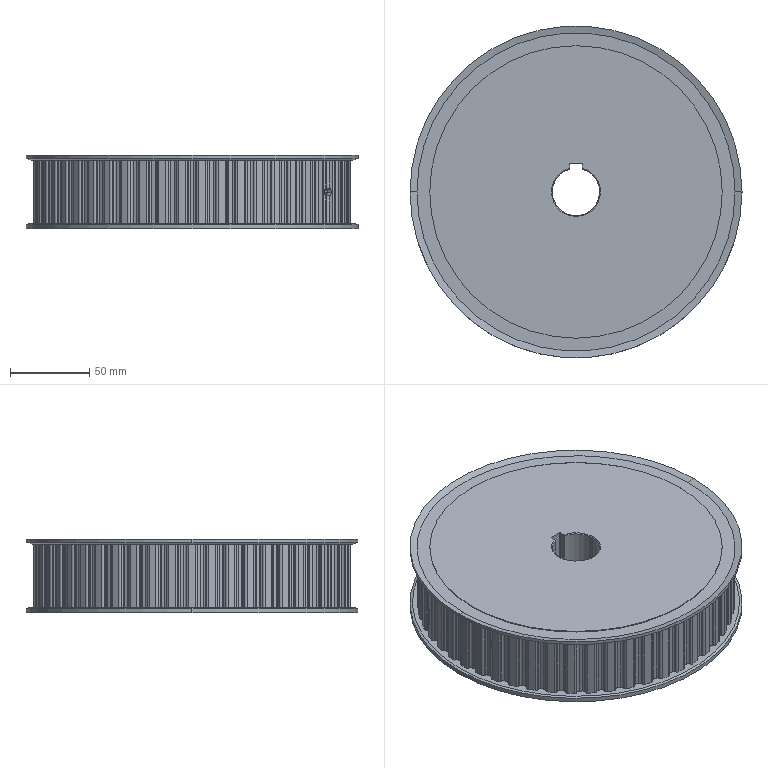Part | SolidWorks | features Revolution 6, ICE 4, RevCut 3, LockFeature 1 | 1 solid | 506 faces | box 210 x 210 x 46.349 mm | volume 1373265 mm3 | cylinder 364 | plane 128 | cone 14 | commonest cylinder face diameters 2.84 x121 2.94 x120 195.58 x51 200.76 x51 4.917 x8 185 x4